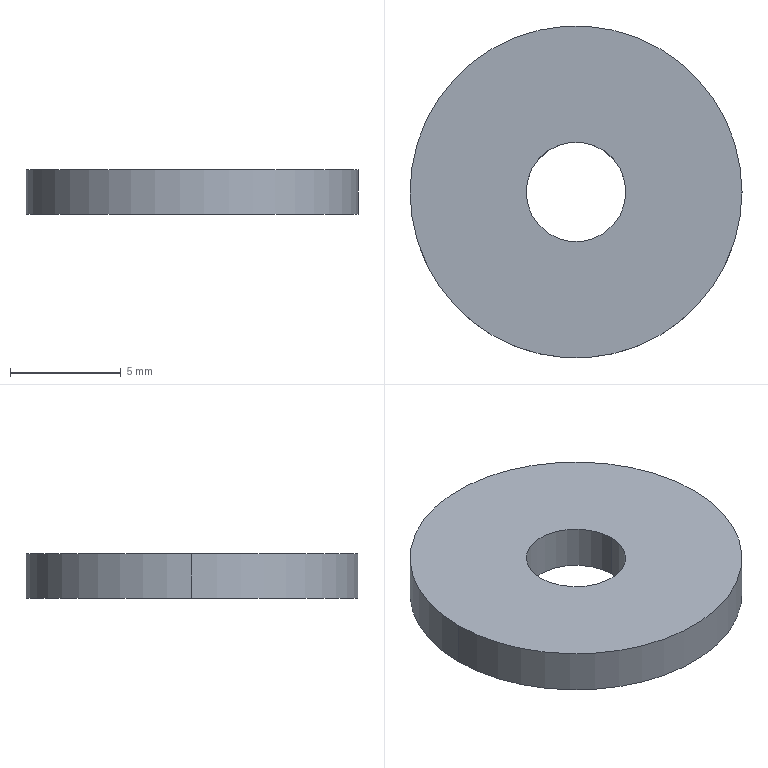Part | SolidWorks | features Extrusion 1 | 1 solid | 6 faces | box 15 x 15 x 2 mm | volume 321.621 mm3 | cylinder 4 | plane 2 | commonest cylinder face diameters 4.5 x2 15 x2
STEP:
#1=CARTESIAN_POINT('',(-2.25,0.,2.));
#2=VERTEX_POINT('',#1);
#3=CARTESIAN_POINT('',(2.25,0.,2.));
#4=VERTEX_POINT('',#3);
#5=CARTESIAN_POINT('',(0.,0.,2.));
#6=DIRECTION('',(0.,0.,1.));
#7=DIRECTION('',(1.,0.,0.));
#8=AXIS2_PLACEMENT_3D('',#5,#6,#7);
#9=CIRCLE('',#8,2.25);
#10=EDGE_CURVE('',#2,#4,#9,.T.);
#11=ORIENTED_EDGE('',*,*,#10,.T.);
#12=CARTESIAN_POINT('',(2.25,0.,0.));
#13=VERTEX_POINT('',#12);
#14=CARTESIAN_POINT('',(2.25,0.,2.));
#15=DIRECTION('',(0.,0.,-1.));
#16=VECTOR('',#15,1000.);
#17=LINE('',#14,#16);
#18=EDGE_CURVE('',#4,#13,#17,.T.);
#19=ORIENTED_EDGE('',*,*,#18,.T.);
#20=CARTESIAN_POINT('',(-2.25,0.,0.));
#21=VERTEX_POINT('',#20);
#22=CARTESIAN_POINT('',(0.,0.,0.));
#23=DIRECTION('',(0.,0.,1.));
#24=DIRECTION('',(1.,0.,0.));
#25=AXIS2_PLACEMENT_3D('',#22,#23,#24);
#26=CIRCLE('',#25,2.25);
#27=EDGE_CURVE('',#21,#13,#26,.T.);
#28=ORIENTED_EDGE('',*,*,#27,.F.);
#29=CARTESIAN_POINT('',(-2.25,0.,2.));
#30=DIRECTION('',(0.,0.,-1.));
#31=VECTOR('',#30,1000.);
#32=LINE('',#29,#31);
#33=EDGE_CURVE('',#2,#21,#32,.T.);
#34=ORIENTED_EDGE('',*,*,#33,.F.);
#35=EDGE_LOOP('',(#11,#19,#28,#34));
#36=FACE_OUTER_BOUND('',#35,.T.);
#37=CARTESIAN_POINT('',(0.,0.,2.));
#38=DIRECTION('',(0.,0.,-1.));
#39=DIRECTION('',(-1.,0.,0.));
#40=AXIS2_PLACEMENT_3D('',#37,#38,#39);
#41=CYLINDRICAL_SURFACE('',#40,2.25);
#42=ADVANCED_FACE('',(#36),#41,.F.);
#43=CARTESIAN_POINT('',(7.5,0.,2.));
#44=VERTEX_POINT('',#43);
#45=CARTESIAN_POINT('',(-7.5,0.,2.));
#46=VERTEX_POINT('',#45);
#47=CARTESIAN_POINT('',(0.,0.,2.));
#48=DIRECTION('',(0.,0.,1.));
#49=DIRECTION('',(1.,0.,0.));
#50=AXIS2_PLACEMENT_3D('',#47,#48,#49);
#51=CIRCLE('',#50,7.5);
#52=EDGE_CURVE('',#44,#46,#51,.T.);
#53=ORIENTED_EDGE('',*,*,#52,.F.);
#54=CARTESIAN_POINT('',(7.5,0.,0.));
#55=VERTEX_POINT('',#54);
#56=CARTESIAN_POINT('',(7.5,0.,2.));
#57=DIRECTION('',(0.,0.,-1.));
#58=VECTOR('',#57,1000.);
#59=LINE('',#56,#58);
#60=EDGE_CURVE('',#44,#55,#59,.T.);
#61=ORIENTED_EDGE('',*,*,#60,.T.);
#62=CARTESIAN_POINT('',(-7.5,0.,0.));
#63=VERTEX_POINT('',#62);
#64=CARTESIAN_POINT('',(0.,0.,0.));
#65=DIRECTION('',(0.,0.,1.));
#66=DIRECTION('',(1.,0.,0.));
#67=AXIS2_PLACEMENT_3D('',#64,#65,#66);
#68=CIRCLE('',#67,7.5);
#69=EDGE_CURVE('',#55,#63,#68,.T.);
#70=ORIENTED_EDGE('',*,*,#69,.T.);
#71=CARTESIAN_POINT('',(-7.5,0.,2.));
#72=DIRECTION('',(0.,0.,-1.));
#73=VECTOR('',#72,1000.);
#74=LINE('',#71,#73);
#75=EDGE_CURVE('',#46,#63,#74,.T.);
#76=ORIENTED_EDGE('',*,*,#75,.F.);
#77=EDGE_LOOP('',(#53,#61,#70,#76));
#78=FACE_OUTER_BOUND('',#77,.T.);
#79=CARTESIAN_POINT('',(0.,0.,2.));
#80=DIRECTION('',(0.,0.,-1.));
#81=DIRECTION('',(-1.,0.,0.));
#82=AXIS2_PLACEMENT_3D('',#79,#80,#81);
#83=CYLINDRICAL_SURFACE('',#82,7.5);
#84=ADVANCED_FACE('',(#78),#83,.T.);
#85=CARTESIAN_POINT('',(0.,0.,2.));
#86=DIRECTION('',(0.,0.,1.));
#87=DIRECTION('',(1.,0.,0.));
#88=AXIS2_PLACEMENT_3D('',#85,#86,#87);
#89=CIRCLE('',#88,7.5);
#90=EDGE_CURVE('',#46,#44,#89,.T.);
#91=ORIENTED_EDGE('',*,*,#90,.T.);
#92=ORIENTED_EDGE('',*,*,#52,.T.);
#93=EDGE_LOOP('',(#91,#92));
#94=FACE_OUTER_BOUND('',#93,.T.);
#95=ORIENTED_EDGE('',*,*,#10,.F.);
#96=CARTESIAN_POINT('',(0.,0.,2.));
#97=DIRECTION('',(0.,0.,1.));
#98=DIRECTION('',(1.,0.,0.));
#99=AXIS2_PLACEMENT_3D('',#96,#97,#98);
#100=CIRCLE('',#99,2.25);
#101=EDGE_CURVE('',#4,#2,#100,.T.);
#102=ORIENTED_EDGE('',*,*,#101,.F.);
#103=EDGE_LOOP('',(#95,#102));
#104=FACE_BOUND('',#103,.T.);
#105=CARTESIAN_POINT('',(0.,0.,2.));
#106=DIRECTION('',(0.,0.,1.));
#107=DIRECTION('',(1.,0.,0.));
#108=AXIS2_PLACEMENT_3D('',#105,#106,#107);
#109=PLANE('',#108);
#110=ADVANCED_FACE('',(#94,#104),#109,.T.);
#111=CARTESIAN_POINT('',(0.,0.,0.));
#112=DIRECTION('',(0.,0.,1.));
#113=DIRECTION('',(1.,0.,0.));
#114=AXIS2_PLACEMENT_3D('',#111,#112,#113);
#115=CIRCLE('',#114,7.5);
#116=EDGE_CURVE('',#63,#55,#115,.T.);
#117=ORIENTED_EDGE('',*,*,#116,.F.);
#118=ORIENTED_EDGE('',*,*,#69,.F.);
#119=EDGE_LOOP('',(#117,#118));
#120=FACE_OUTER_BOUND('',#119,.T.);
#121=ORIENTED_EDGE('',*,*,#27,.T.);
#122=CARTESIAN_POINT('',(0.,0.,0.));
#123=DIRECTION('',(0.,0.,1.));
#124=DIRECTION('',(1.,0.,0.));
#125=AXIS2_PLACEMENT_3D('',#122,#123,#124);
#126=CIRCLE('',#125,2.25);
#127=EDGE_CURVE('',#13,#21,#126,.T.);
#128=ORIENTED_EDGE('',*,*,#127,.T.);
#129=EDGE_LOOP('',(#121,#128));
#130=FACE_BOUND('',#129,.T.);
#131=CARTESIAN_POINT('',(0.,0.,0.));
#132=DIRECTION('',(0.,0.,1.));
#133=DIRECTION('',(1.,0.,0.));
#134=AXIS2_PLACEMENT_3D('',#131,#132,#133);
#135=PLANE('',#134);
#136=ADVANCED_FACE('',(#120,#130),#135,.F.);
#137=ORIENTED_EDGE('',*,*,#60,.F.);
#138=ORIENTED_EDGE('',*,*,#90,.F.);
#139=ORIENTED_EDGE('',*,*,#75,.T.);
#140=ORIENTED_EDGE('',*,*,#116,.T.);
#141=EDGE_LOOP('',(#137,#138,#139,#140));
#142=FACE_OUTER_BOUND('',#141,.T.);
#143=CARTESIAN_POINT('',(0.,0.,2.));
#144=DIRECTION('',(0.,0.,-1.));
#145=DIRECTION('',(-1.,0.,0.));
#146=AXIS2_PLACEMENT_3D('',#143,#144,#145);
#147=CYLINDRICAL_SURFACE('',#146,7.5);
#148=ADVANCED_FACE('',(#142),#147,.T.);
#149=ORIENTED_EDGE('',*,*,#18,.F.);
#150=ORIENTED_EDGE('',*,*,#101,.T.);
#151=ORIENTED_EDGE('',*,*,#33,.T.);
#152=ORIENTED_EDGE('',*,*,#127,.F.);
#153=EDGE_LOOP('',(#149,#150,#151,#152));
#154=FACE_OUTER_BOUND('',#153,.T.);
#155=CARTESIAN_POINT('',(0.,0.,2.));
#156=DIRECTION('',(0.,0.,-1.));
#157=DIRECTION('',(-1.,0.,0.));
#158=AXIS2_PLACEMENT_3D('',#155,#156,#157);
#159=CYLINDRICAL_SURFACE('',#158,2.25);
#160=ADVANCED_FACE('',(#154),#159,.F.);
#161=CLOSED_SHELL('',(#42,#84,#110,#136,#148,#160));
#162=MANIFOLD_SOLID_BREP('',#161);
#163=CARTESIAN_POINT('',(0.,0.,0.));
#164=DIRECTION('',(0.,0.,1.));
#165=DIRECTION('',(1.,0.,0.));
#166=AXIS2_PLACEMENT_3D('',#163,#164,#165);
#167=(LENGTH_UNIT()NAMED_UNIT(*)SI_UNIT(.MILLI.,.METRE.));
#168=UNCERTAINTY_MEASURE_WITH_UNIT(LENGTH_MEASURE(0.00001),#167,'','');
#169=(NAMED_UNIT(*)PLANE_ANGLE_UNIT()SI_UNIT($,.RADIAN.));
#170=(NAMED_UNIT(*)SI_UNIT($,.STERADIAN.)SOLID_ANGLE_UNIT());
#171=(GEOMETRIC_REPRESENTATION_CONTEXT(3)GLOBAL_UNCERTAINTY_ASSIGNED_CONTEXT((#168))GLOBAL_UNIT_ASSIGNED_CONTEXT((#167,#169,#170))REPRESENTATION_CONTEXT('',''));
#172=ADVANCED_BREP_SHAPE_REPRESENTATION('',(#162,#166),#171);